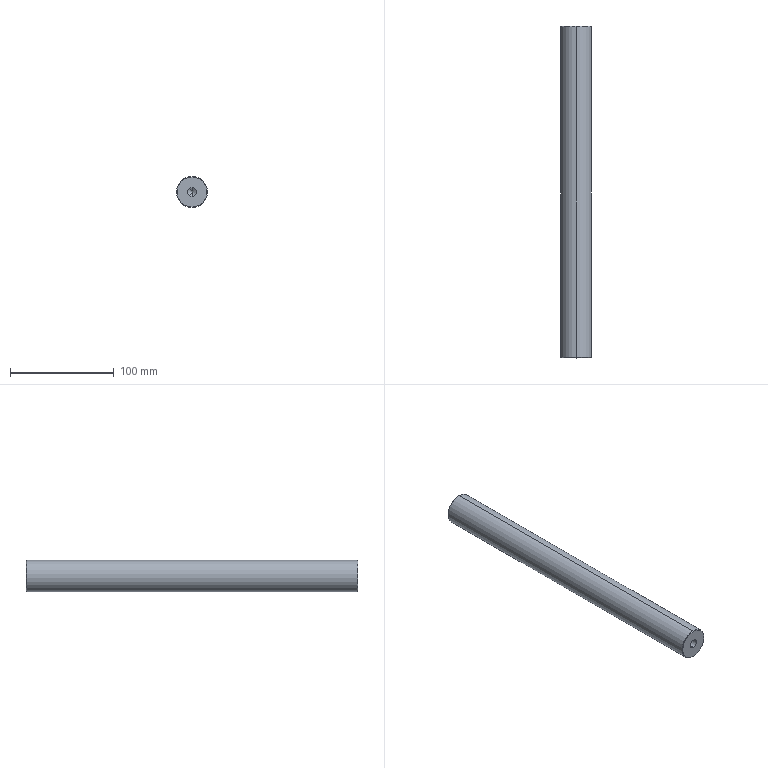Part | SolidWorks | features HoleWzd 2, Chamfer 1, Extrusion 1 | 1 solid | 16 faces | box 30 x 320 x 30 mm | volume 223294 mm3 | cone 8 | cylinder 6 | plane 2 | commonest cylinder face diameters 8.5 x4 30 x2
STEP:
#1=CARTESIAN_POINT('',(0.,-135.5,4.25));
#2=VERTEX_POINT('',#1);
#3=CARTESIAN_POINT('',(0.,-135.5,-4.25));
#4=VERTEX_POINT('',#3);
#5=CARTESIAN_POINT('',(0.,-135.5,0.));
#6=DIRECTION('',(0.,-1.,0.));
#7=DIRECTION('',(0.,0.,-1.));
#8=AXIS2_PLACEMENT_3D('',#5,#6,#7);
#9=CIRCLE('',#8,4.25);
#10=EDGE_CURVE('',#2,#4,#9,.T.);
#11=ORIENTED_EDGE('',*,*,#10,.F.);
#12=CARTESIAN_POINT('',(0.,-160.,4.25));
#13=VERTEX_POINT('',#12);
#14=CARTESIAN_POINT('',(0.,-160.,4.25));
#15=DIRECTION('',(0.,-1.,0.));
#16=VECTOR('',#15,1000.);
#17=LINE('',#14,#16);
#18=EDGE_CURVE('',#2,#13,#17,.T.);
#19=ORIENTED_EDGE('',*,*,#18,.T.);
#20=CARTESIAN_POINT('',(0.,-160.,-4.25));
#21=VERTEX_POINT('',#20);
#22=CARTESIAN_POINT('',(0.,-160.,0.));
#23=DIRECTION('',(0.,-1.,0.));
#24=DIRECTION('',(0.,0.,-1.));
#25=AXIS2_PLACEMENT_3D('',#22,#23,#24);
#26=CIRCLE('',#25,4.25);
#27=EDGE_CURVE('',#13,#21,#26,.T.);
#28=ORIENTED_EDGE('',*,*,#27,.T.);
#29=CARTESIAN_POINT('',(0.,-160.,-4.25));
#30=DIRECTION('',(0.,-1.,0.));
#31=VECTOR('',#30,1000.);
#32=LINE('',#29,#31);
#33=EDGE_CURVE('',#4,#21,#32,.T.);
#34=ORIENTED_EDGE('',*,*,#33,.F.);
#35=EDGE_LOOP('',(#11,#19,#28,#34));
#36=FACE_OUTER_BOUND('',#35,.T.);
#37=CARTESIAN_POINT('',(0.,-160.,0.));
#38=DIRECTION('',(0.,-1.,0.));
#39=DIRECTION('',(0.,0.,-1.));
#40=AXIS2_PLACEMENT_3D('',#37,#38,#39);
#41=CYLINDRICAL_SURFACE('',#40,4.25);
#42=ADVANCED_FACE('',(#36),#41,.F.);
#43=CARTESIAN_POINT('',(0.,-132.946,0.));
#44=VERTEX_POINT('',#43);
#45=CARTESIAN_POINT('',(0.,-135.5,-4.25));
#46=DIRECTION('',(0.,-0.515,-0.8572));
#47=VECTOR('',#46,1000.);
#48=LINE('',#45,#47);
#49=EDGE_CURVE('',#44,#4,#48,.T.);
#50=ORIENTED_EDGE('',*,*,#49,.F.);
#51=CARTESIAN_POINT('',(0.,-135.5,4.25));
#52=DIRECTION('',(0.,-0.515,0.8572));
#53=VECTOR('',#52,1000.);
#54=LINE('',#51,#53);
#55=EDGE_CURVE('',#44,#2,#54,.T.);
#56=ORIENTED_EDGE('',*,*,#55,.T.);
#57=ORIENTED_EDGE('',*,*,#10,.T.);
#58=EDGE_LOOP('',(#50,#56,#57));
#59=FACE_OUTER_BOUND('',#58,.T.);
#60=CARTESIAN_POINT('',(0.,-135.5,0.));
#61=DIRECTION('',(0.,-1.,0.));
#62=DIRECTION('',(0.,0.,-1.));
#63=AXIS2_PLACEMENT_3D('',#60,#61,#62);
#64=CONICAL_SURFACE('',#63,4.25,1.03);
#65=ADVANCED_FACE('',(#59),#64,.F.);
#66=CARTESIAN_POINT('',(0.,135.5,-4.25));
#67=VERTEX_POINT('',#66);
#68=CARTESIAN_POINT('',(0.,135.5,4.25));
#69=VERTEX_POINT('',#68);
#70=CARTESIAN_POINT('',(0.,135.5,0.));
#71=DIRECTION('',(0.,1.,0.));
#72=DIRECTION('',(0.,0.,1.));
#73=AXIS2_PLACEMENT_3D('',#70,#71,#72);
#74=CIRCLE('',#73,4.25);
#75=EDGE_CURVE('',#67,#69,#74,.T.);
#76=ORIENTED_EDGE('',*,*,#75,.F.);
#77=CARTESIAN_POINT('',(0.,160.,-4.25));
#78=VERTEX_POINT('',#77);
#79=CARTESIAN_POINT('',(0.,160.,-4.25));
#80=DIRECTION('',(0.,1.,0.));
#81=VECTOR('',#80,1000.);
#82=LINE('',#79,#81);
#83=EDGE_CURVE('',#67,#78,#82,.T.);
#84=ORIENTED_EDGE('',*,*,#83,.T.);
#85=CARTESIAN_POINT('',(0.,160.,4.25));
#86=VERTEX_POINT('',#85);
#87=CARTESIAN_POINT('',(0.,160.,0.));
#88=DIRECTION('',(0.,1.,0.));
#89=DIRECTION('',(0.,0.,1.));
#90=AXIS2_PLACEMENT_3D('',#87,#88,#89);
#91=CIRCLE('',#90,4.25);
#92=EDGE_CURVE('',#78,#86,#91,.T.);
#93=ORIENTED_EDGE('',*,*,#92,.T.);
#94=CARTESIAN_POINT('',(0.,160.,4.25));
#95=DIRECTION('',(0.,1.,0.));
#96=VECTOR('',#95,1000.);
#97=LINE('',#94,#96);
#98=EDGE_CURVE('',#69,#86,#97,.T.);
#99=ORIENTED_EDGE('',*,*,#98,.F.);
#100=EDGE_LOOP('',(#76,#84,#93,#99));
#101=FACE_OUTER_BOUND('',#100,.T.);
#102=CARTESIAN_POINT('',(0.,160.,0.));
#103=DIRECTION('',(0.,1.,0.));
#104=DIRECTION('',(0.,0.,1.));
#105=AXIS2_PLACEMENT_3D('',#102,#103,#104);
#106=CYLINDRICAL_SURFACE('',#105,4.25);
#107=ADVANCED_FACE('',(#101),#106,.F.);
#108=CARTESIAN_POINT('',(0.,132.946,0.));
#109=VERTEX_POINT('',#108);
#110=CARTESIAN_POINT('',(0.,135.5,4.25));
#111=DIRECTION('',(0.,0.515,0.8572));
#112=VECTOR('',#111,1000.);
#113=LINE('',#110,#112);
#114=EDGE_CURVE('',#109,#69,#113,.T.);
#115=ORIENTED_EDGE('',*,*,#114,.F.);
#116=CARTESIAN_POINT('',(0.,135.5,-4.25));
#117=DIRECTION('',(0.,0.515,-0.8572));
#118=VECTOR('',#117,1000.);
#119=LINE('',#116,#118);
#120=EDGE_CURVE('',#109,#67,#119,.T.);
#121=ORIENTED_EDGE('',*,*,#120,.T.);
#122=ORIENTED_EDGE('',*,*,#75,.T.);
#123=EDGE_LOOP('',(#115,#121,#122));
#124=FACE_OUTER_BOUND('',#123,.T.);
#125=CARTESIAN_POINT('',(0.,135.5,0.));
#126=DIRECTION('',(0.,1.,0.));
#127=DIRECTION('',(0.,0.,1.));
#128=AXIS2_PLACEMENT_3D('',#125,#126,#127);
#129=CONICAL_SURFACE('',#128,4.25,1.03);
#130=ADVANCED_FACE('',(#124),#129,.F.);
#131=CARTESIAN_POINT('',(0.,160.,14.5));
#132=VERTEX_POINT('',#131);
#133=CARTESIAN_POINT('',(0.,160.,-14.5));
#134=VERTEX_POINT('',#133);
#135=CARTESIAN_POINT('',(0.,160.,0.));
#136=DIRECTION('',(0.,1.,0.));
#137=DIRECTION('',(0.,0.,1.));
#138=AXIS2_PLACEMENT_3D('',#135,#136,#137);
#139=CIRCLE('',#138,14.5);
#140=EDGE_CURVE('',#132,#134,#139,.T.);
#141=ORIENTED_EDGE('',*,*,#140,.F.);
#142=CARTESIAN_POINT('',(0.,159.5,15.));
#143=VERTEX_POINT('',#142);
#144=CARTESIAN_POINT('',(0.,160.,14.5));
#145=DIRECTION('',(0.,-0.7071,0.7071));
#146=VECTOR('',#145,1000.);
#147=LINE('',#144,#146);
#148=EDGE_CURVE('',#132,#143,#147,.T.);
#149=ORIENTED_EDGE('',*,*,#148,.T.);
#150=CARTESIAN_POINT('',(0.,159.5,-15.));
#151=VERTEX_POINT('',#150);
#152=CARTESIAN_POINT('',(0.,159.5,0.));
#153=DIRECTION('',(0.,-1.,0.));
#154=DIRECTION('',(0.,0.,1.));
#155=AXIS2_PLACEMENT_3D('',#152,#153,#154);
#156=CIRCLE('',#155,15.);
#157=EDGE_CURVE('',#151,#143,#156,.T.);
#158=ORIENTED_EDGE('',*,*,#157,.F.);
#159=CARTESIAN_POINT('',(0.,160.,-14.5));
#160=DIRECTION('',(0.,-0.7071,-0.7071));
#161=VECTOR('',#160,1000.);
#162=LINE('',#159,#161);
#163=EDGE_CURVE('',#134,#151,#162,.T.);
#164=ORIENTED_EDGE('',*,*,#163,.F.);
#165=EDGE_LOOP('',(#141,#149,#158,#164));
#166=FACE_OUTER_BOUND('',#165,.T.);
#167=CARTESIAN_POINT('',(0.,160.,0.));
#168=DIRECTION('',(0.,-1.,0.));
#169=DIRECTION('',(0.,0.,-1.));
#170=AXIS2_PLACEMENT_3D('',#167,#168,#169);
#171=CONICAL_SURFACE('',#170,14.5,0.7854);
#172=ADVANCED_FACE('',(#166),#171,.T.);
#173=CARTESIAN_POINT('',(0.,-160.,-14.5));
#174=VERTEX_POINT('',#173);
#175=CARTESIAN_POINT('',(0.,-160.,14.5));
#176=VERTEX_POINT('',#175);
#177=CARTESIAN_POINT('',(0.,-160.,0.));
#178=DIRECTION('',(0.,-1.,0.));
#179=DIRECTION('',(0.,0.,1.));
#180=AXIS2_PLACEMENT_3D('',#177,#178,#179);
#181=CIRCLE('',#180,14.5);
#182=EDGE_CURVE('',#174,#176,#181,.T.);
#183=ORIENTED_EDGE('',*,*,#182,.F.);
#184=CARTESIAN_POINT('',(0.,-159.5,-15.));
#185=VERTEX_POINT('',#184);
#186=CARTESIAN_POINT('',(0.,-159.5,-15.));
#187=DIRECTION('',(0.,0.7071,-0.7071));
#188=VECTOR('',#187,1000.);
#189=LINE('',#186,#188);
#190=EDGE_CURVE('',#174,#185,#189,.T.);
#191=ORIENTED_EDGE('',*,*,#190,.T.);
#192=CARTESIAN_POINT('',(0.,-159.5,15.));
#193=VERTEX_POINT('',#192);
#194=CARTESIAN_POINT('',(0.,-159.5,0.));
#195=DIRECTION('',(0.,1.,0.));
#196=DIRECTION('',(0.,0.,1.));
#197=AXIS2_PLACEMENT_3D('',#194,#195,#196);
#198=CIRCLE('',#197,15.);
#199=EDGE_CURVE('',#193,#185,#198,.T.);
#200=ORIENTED_EDGE('',*,*,#199,.F.);
#201=CARTESIAN_POINT('',(0.,-159.5,15.));
#202=DIRECTION('',(0.,0.7071,0.7071));
#203=VECTOR('',#202,1000.);
#204=LINE('',#201,#203);
#205=EDGE_CURVE('',#176,#193,#204,.T.);
#206=ORIENTED_EDGE('',*,*,#205,.F.);
#207=EDGE_LOOP('',(#183,#191,#200,#206));
#208=FACE_OUTER_BOUND('',#207,.T.);
#209=CARTESIAN_POINT('',(0.,-159.5,0.));
#210=DIRECTION('',(0.,1.,0.));
#211=DIRECTION('',(0.,0.,1.));
#212=AXIS2_PLACEMENT_3D('',#209,#210,#211);
#213=CONICAL_SURFACE('',#212,15.,0.7854);
#214=ADVANCED_FACE('',(#208),#213,.T.);
#215=ORIENTED_EDGE('',*,*,#157,.T.);
#216=CARTESIAN_POINT('',(0.,160.,15.));
#217=DIRECTION('',(0.,-1.,0.));
#218=VECTOR('',#217,1000.);
#219=LINE('',#216,#218);
#220=EDGE_CURVE('',#143,#193,#219,.T.);
#221=ORIENTED_EDGE('',*,*,#220,.T.);
#222=ORIENTED_EDGE('',*,*,#199,.T.);
#223=CARTESIAN_POINT('',(0.,160.,-15.));
#224=DIRECTION('',(0.,-1.,0.));
#225=VECTOR('',#224,1000.);
#226=LINE('',#223,#225);
#227=EDGE_CURVE('',#151,#185,#226,.T.);
#228=ORIENTED_EDGE('',*,*,#227,.F.);
#229=EDGE_LOOP('',(#215,#221,#222,#228));
#230=FACE_OUTER_BOUND('',#229,.T.);
#231=CARTESIAN_POINT('',(0.,160.,0.));
#232=DIRECTION('',(0.,-1.,0.));
#233=DIRECTION('',(0.,0.,-1.));
#234=AXIS2_PLACEMENT_3D('',#231,#232,#233);
#235=CYLINDRICAL_SURFACE('',#234,15.);
#236=ADVANCED_FACE('',(#230),#235,.T.);
#237=ORIENTED_EDGE('',*,*,#220,.F.);
#238=CARTESIAN_POINT('',(0.,159.5,0.));
#239=DIRECTION('',(0.,-1.,0.));
#240=DIRECTION('',(0.,0.,1.));
#241=AXIS2_PLACEMENT_3D('',#238,#239,#240);
#242=CIRCLE('',#241,15.);
#243=EDGE_CURVE('',#143,#151,#242,.T.);
#244=ORIENTED_EDGE('',*,*,#243,.T.);
#245=ORIENTED_EDGE('',*,*,#227,.T.);
#246=CARTESIAN_POINT('',(0.,-159.5,0.));
#247=DIRECTION('',(0.,1.,0.));
#248=DIRECTION('',(0.,0.,1.));
#249=AXIS2_PLACEMENT_3D('',#246,#247,#248);
#250=CIRCLE('',#249,15.);
#251=EDGE_CURVE('',#185,#193,#250,.T.);
#252=ORIENTED_EDGE('',*,*,#251,.T.);
#253=EDGE_LOOP('',(#237,#244,#245,#252));
#254=FACE_OUTER_BOUND('',#253,.T.);
#255=CARTESIAN_POINT('',(0.,160.,0.));
#256=DIRECTION('',(0.,-1.,0.));
#257=DIRECTION('',(0.,0.,-1.));
#258=AXIS2_PLACEMENT_3D('',#255,#256,#257);
#259=CYLINDRICAL_SURFACE('',#258,15.);
#260=ADVANCED_FACE('',(#254),#259,.T.);
#261=CARTESIAN_POINT('',(0.,160.,0.));
#262=DIRECTION('',(0.,1.,0.));
#263=DIRECTION('',(0.,0.,1.));
#264=AXIS2_PLACEMENT_3D('',#261,#262,#263);
#265=CIRCLE('',#264,4.25);
#266=EDGE_CURVE('',#86,#78,#265,.T.);
#267=ORIENTED_EDGE('',*,*,#266,.F.);
#268=ORIENTED_EDGE('',*,*,#92,.F.);
#269=EDGE_LOOP('',(#267,#268));
#270=FACE_BOUND('',#269,.T.);
#271=CARTESIAN_POINT('',(0.,160.,0.));
#272=DIRECTION('',(0.,1.,0.));
#273=DIRECTION('',(0.,0.,1.));
#274=AXIS2_PLACEMENT_3D('',#271,#272,#273);
#275=CIRCLE('',#274,14.5);
#276=EDGE_CURVE('',#134,#132,#275,.T.);
#277=ORIENTED_EDGE('',*,*,#276,.T.);
#278=ORIENTED_EDGE('',*,*,#140,.T.);
#279=EDGE_LOOP('',(#277,#278));
#280=FACE_OUTER_BOUND('',#279,.T.);
#281=CARTESIAN_POINT('',(0.,160.,0.));
#282=DIRECTION('',(0.,1.,0.));
#283=DIRECTION('',(0.,0.,1.));
#284=AXIS2_PLACEMENT_3D('',#281,#282,#283);
#285=PLANE('',#284);
#286=ADVANCED_FACE('',(#270,#280),#285,.T.);
#287=CARTESIAN_POINT('',(0.,-160.,0.));
#288=DIRECTION('',(0.,-1.,0.));
#289=DIRECTION('',(0.,0.,-1.));
#290=AXIS2_PLACEMENT_3D('',#287,#288,#289);
#291=CIRCLE('',#290,4.25);
#292=EDGE_CURVE('',#21,#13,#291,.T.);
#293=ORIENTED_EDGE('',*,*,#292,.F.);
#294=ORIENTED_EDGE('',*,*,#27,.F.);
#295=EDGE_LOOP('',(#293,#294));
#296=FACE_BOUND('',#295,.T.);
#297=CARTESIAN_POINT('',(0.,-160.,0.));
#298=DIRECTION('',(0.,-1.,0.));
#299=DIRECTION('',(0.,0.,1.));
#300=AXIS2_PLACEMENT_3D('',#297,#298,#299);
#301=CIRCLE('',#300,14.5);
#302=EDGE_CURVE('',#176,#174,#301,.T.);
#303=ORIENTED_EDGE('',*,*,#302,.T.);
#304=ORIENTED_EDGE('',*,*,#182,.T.);
#305=EDGE_LOOP('',(#303,#304));
#306=FACE_OUTER_BOUND('',#305,.T.);
#307=CARTESIAN_POINT('',(0.,-160.,0.));
#308=DIRECTION('',(0.,1.,0.));
#309=DIRECTION('',(0.,0.,1.));
#310=AXIS2_PLACEMENT_3D('',#307,#308,#309);
#311=PLANE('',#310);
#312=ADVANCED_FACE('',(#296,#306),#311,.F.);
#313=ORIENTED_EDGE('',*,*,#190,.F.);
#314=ORIENTED_EDGE('',*,*,#302,.F.);
#315=ORIENTED_EDGE('',*,*,#205,.T.);
#316=ORIENTED_EDGE('',*,*,#251,.F.);
#317=EDGE_LOOP('',(#313,#314,#315,#316));
#318=FACE_OUTER_BOUND('',#317,.T.);
#319=CARTESIAN_POINT('',(0.,-159.5,0.));
#320=DIRECTION('',(0.,1.,0.));
#321=DIRECTION('',(0.,0.,1.));
#322=AXIS2_PLACEMENT_3D('',#319,#320,#321);
#323=CONICAL_SURFACE('',#322,15.,0.7854);
#324=ADVANCED_FACE('',(#318),#323,.T.);
#325=ORIENTED_EDGE('',*,*,#148,.F.);
#326=ORIENTED_EDGE('',*,*,#276,.F.);
#327=ORIENTED_EDGE('',*,*,#163,.T.);
#328=ORIENTED_EDGE('',*,*,#243,.F.);
#329=EDGE_LOOP('',(#325,#326,#327,#328));
#330=FACE_OUTER_BOUND('',#329,.T.);
#331=CARTESIAN_POINT('',(0.,160.,0.));
#332=DIRECTION('',(0.,-1.,0.));
#333=DIRECTION('',(0.,0.,-1.));
#334=AXIS2_PLACEMENT_3D('',#331,#332,#333);
#335=CONICAL_SURFACE('',#334,14.5,0.7854);
#336=ADVANCED_FACE('',(#330),#335,.T.);
#337=ORIENTED_EDGE('',*,*,#120,.F.);
#338=ORIENTED_EDGE('',*,*,#114,.T.);
#339=CARTESIAN_POINT('',(0.,135.5,0.));
#340=DIRECTION('',(0.,1.,0.));
#341=DIRECTION('',(0.,0.,1.));
#342=AXIS2_PLACEMENT_3D('',#339,#340,#341);
#343=CIRCLE('',#342,4.25);
#344=EDGE_CURVE('',#69,#67,#343,.T.);
#345=ORIENTED_EDGE('',*,*,#344,.T.);
#346=EDGE_LOOP('',(#337,#338,#345));
#347=FACE_OUTER_BOUND('',#346,.T.);
#348=CARTESIAN_POINT('',(0.,135.5,0.));
#349=DIRECTION('',(0.,1.,0.));
#350=DIRECTION('',(0.,0.,1.));
#351=AXIS2_PLACEMENT_3D('',#348,#349,#350);
#352=CONICAL_SURFACE('',#351,4.25,1.03);
#353=ADVANCED_FACE('',(#347),#352,.F.);
#354=ORIENTED_EDGE('',*,*,#83,.F.);
#355=ORIENTED_EDGE('',*,*,#344,.F.);
#356=ORIENTED_EDGE('',*,*,#98,.T.);
#357=ORIENTED_EDGE('',*,*,#266,.T.);
#358=EDGE_LOOP('',(#354,#355,#356,#357));
#359=FACE_OUTER_BOUND('',#358,.T.);
#360=CARTESIAN_POINT('',(0.,160.,0.));
#361=DIRECTION('',(0.,1.,0.));
#362=DIRECTION('',(0.,0.,1.));
#363=AXIS2_PLACEMENT_3D('',#360,#361,#362);
#364=CYLINDRICAL_SURFACE('',#363,4.25);
#365=ADVANCED_FACE('',(#359),#364,.F.);
#366=ORIENTED_EDGE('',*,*,#55,.F.);
#367=ORIENTED_EDGE('',*,*,#49,.T.);
#368=CARTESIAN_POINT('',(0.,-135.5,0.));
#369=DIRECTION('',(0.,-1.,0.));
#370=DIRECTION('',(0.,0.,-1.));
#371=AXIS2_PLACEMENT_3D('',#368,#369,#370);
#372=CIRCLE('',#371,4.25);
#373=EDGE_CURVE('',#4,#2,#372,.T.);
#374=ORIENTED_EDGE('',*,*,#373,.T.);
#375=EDGE_LOOP('',(#366,#367,#374));
#376=FACE_OUTER_BOUND('',#375,.T.);
#377=CARTESIAN_POINT('',(0.,-135.5,0.));
#378=DIRECTION('',(0.,-1.,0.));
#379=DIRECTION('',(0.,0.,-1.));
#380=AXIS2_PLACEMENT_3D('',#377,#378,#379);
#381=CONICAL_SURFACE('',#380,4.25,1.03);
#382=ADVANCED_FACE('',(#376),#381,.F.);
#383=ORIENTED_EDGE('',*,*,#18,.F.);
#384=ORIENTED_EDGE('',*,*,#373,.F.);
#385=ORIENTED_EDGE('',*,*,#33,.T.);
#386=ORIENTED_EDGE('',*,*,#292,.T.);
#387=EDGE_LOOP('',(#383,#384,#385,#386));
#388=FACE_OUTER_BOUND('',#387,.T.);
#389=CARTESIAN_POINT('',(0.,-160.,0.));
#390=DIRECTION('',(0.,-1.,0.));
#391=DIRECTION('',(0.,0.,-1.));
#392=AXIS2_PLACEMENT_3D('',#389,#390,#391);
#393=CYLINDRICAL_SURFACE('',#392,4.25);
#394=ADVANCED_FACE('',(#388),#393,.F.);
#395=CLOSED_SHELL('',(#42,#65,#107,#130,#172,#214,#236,#260,#286,#312,#324,#336,#353,#365,#382,#394));
#396=MANIFOLD_SOLID_BREP('',#395);
#397=CARTESIAN_POINT('',(0.,0.,0.));
#398=DIRECTION('',(0.,0.,1.));
#399=DIRECTION('',(1.,0.,0.));
#400=AXIS2_PLACEMENT_3D('',#397,#398,#399);
#401=(LENGTH_UNIT()NAMED_UNIT(*)SI_UNIT(.MILLI.,.METRE.));
#402=UNCERTAINTY_MEASURE_WITH_UNIT(LENGTH_MEASURE(0.00001),#401,'','');
#403=(NAMED_UNIT(*)PLANE_ANGLE_UNIT()SI_UNIT($,.RADIAN.));
#404=(NAMED_UNIT(*)SI_UNIT($,.STERADIAN.)SOLID_ANGLE_UNIT());
#405=(GEOMETRIC_REPRESENTATION_CONTEXT(3)GLOBAL_UNCERTAINTY_ASSIGNED_CONTEXT((#402))GLOBAL_UNIT_ASSIGNED_CONTEXT((#401,#403,#404))REPRESENTATION_CONTEXT('',''));
#406=ADVANCED_BREP_SHAPE_REPRESENTATION('',(#396,#400),#405);